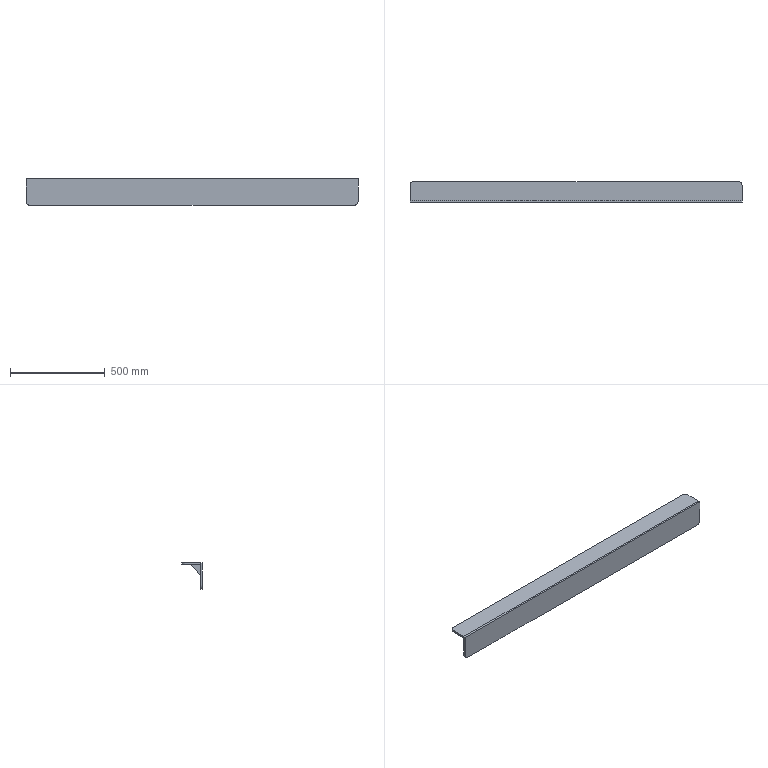Part | SolidWorks | features Fillet 2, ICE 2, Extrusion 1 | 3 solids | 21 faces | box 1748 x 110 x 139.4 mm | volume 4195006 mm3 | plane 17 | cylinder 4 | commonest cylinder face diameters 40 x4
STEP:
#1=CARTESIAN_POINT('',(873.75,0.,69.7));
#2=VERTEX_POINT('',#1);
#3=CARTESIAN_POINT('',(873.75,0.,-49.7));
#4=VERTEX_POINT('',#3);
#5=CARTESIAN_POINT('',(873.75,0.,-69.7));
#6=DIRECTION('',(0.,0.,-1.));
#7=VECTOR('',#6,1000.);
#8=LINE('',#5,#7);
#9=EDGE_CURVE('',#2,#4,#8,.T.);
#10=ORIENTED_EDGE('',*,*,#9,.T.);
#11=CARTESIAN_POINT('',(873.75,10.,-49.7));
#12=VERTEX_POINT('',#11);
#13=CARTESIAN_POINT('',(873.75,10.,-49.7));
#14=DIRECTION('',(0.,1.,0.));
#15=VECTOR('',#14,1000.);
#16=LINE('',#13,#15);
#17=EDGE_CURVE('',#4,#12,#16,.T.);
#18=ORIENTED_EDGE('',*,*,#17,.T.);
#19=CARTESIAN_POINT('',(873.75,10.,69.7));
#20=VERTEX_POINT('',#19);
#21=CARTESIAN_POINT('',(873.75,10.,-69.7));
#22=DIRECTION('',(0.,0.,-1.));
#23=VECTOR('',#22,1000.);
#24=LINE('',#21,#23);
#25=EDGE_CURVE('',#20,#12,#24,.T.);
#26=ORIENTED_EDGE('',*,*,#25,.F.);
#27=CARTESIAN_POINT('',(873.75,10.,69.7));
#28=DIRECTION('',(0.,-1.,0.));
#29=VECTOR('',#28,1000.);
#30=LINE('',#27,#29);
#31=EDGE_CURVE('',#20,#2,#30,.T.);
#32=ORIENTED_EDGE('',*,*,#31,.T.);
#33=EDGE_LOOP('',(#10,#18,#26,#32));
#34=FACE_OUTER_BOUND('',#33,.T.);
#35=CARTESIAN_POINT('',(873.75,10.,-69.7));
#36=DIRECTION('',(-1.,0.,0.));
#37=DIRECTION('',(0.,0.,1.));
#38=AXIS2_PLACEMENT_3D('',#35,#36,#37);
#39=PLANE('',#38);
#40=ADVANCED_FACE('',(#34),#39,.F.);
#41=CARTESIAN_POINT('',(853.75,0.,-69.7));
#42=VERTEX_POINT('',#41);
#43=CARTESIAN_POINT('',(-853.75,0.,-69.7));
#44=VERTEX_POINT('',#43);
#45=CARTESIAN_POINT('',(-873.75,0.,-69.7));
#46=DIRECTION('',(-1.,0.,0.));
#47=VECTOR('',#46,1000.);
#48=LINE('',#45,#47);
#49=EDGE_CURVE('',#42,#44,#48,.T.);
#50=ORIENTED_EDGE('',*,*,#49,.T.);
#51=CARTESIAN_POINT('',(-853.75,10.,-69.7));
#52=VERTEX_POINT('',#51);
#53=CARTESIAN_POINT('',(-853.75,10.,-69.7));
#54=DIRECTION('',(0.,1.,0.));
#55=VECTOR('',#54,1000.);
#56=LINE('',#53,#55);
#57=EDGE_CURVE('',#44,#52,#56,.T.);
#58=ORIENTED_EDGE('',*,*,#57,.T.);
#59=CARTESIAN_POINT('',(853.75,10.,-69.7));
#60=VERTEX_POINT('',#59);
#61=CARTESIAN_POINT('',(-873.75,10.,-69.7));
#62=DIRECTION('',(-1.,0.,0.));
#63=VECTOR('',#62,1000.);
#64=LINE('',#61,#63);
#65=EDGE_CURVE('',#60,#52,#64,.T.);
#66=ORIENTED_EDGE('',*,*,#65,.F.);
#67=CARTESIAN_POINT('',(853.75,10.,-69.7));
#68=DIRECTION('',(0.,-1.,0.));
#69=VECTOR('',#68,1000.);
#70=LINE('',#67,#69);
#71=EDGE_CURVE('',#60,#42,#70,.T.);
#72=ORIENTED_EDGE('',*,*,#71,.T.);
#73=EDGE_LOOP('',(#50,#58,#66,#72));
#74=FACE_OUTER_BOUND('',#73,.T.);
#75=CARTESIAN_POINT('',(-873.75,10.,-69.7));
#76=DIRECTION('',(0.,0.,1.));
#77=DIRECTION('',(1.,0.,0.));
#78=AXIS2_PLACEMENT_3D('',#75,#76,#77);
#79=PLANE('',#78);
#80=ADVANCED_FACE('',(#74),#79,.F.);
#81=CARTESIAN_POINT('',(-873.75,10.,-49.7));
#82=VERTEX_POINT('',#81);
#83=CARTESIAN_POINT('',(-873.75,10.,69.7));
#84=VERTEX_POINT('',#83);
#85=CARTESIAN_POINT('',(-873.75,10.,-69.7));
#86=DIRECTION('',(0.,0.,1.));
#87=VECTOR('',#86,1000.);
#88=LINE('',#85,#87);
#89=EDGE_CURVE('',#82,#84,#88,.T.);
#90=ORIENTED_EDGE('',*,*,#89,.F.);
#91=CARTESIAN_POINT('',(-873.75,0.,-49.7));
#92=VERTEX_POINT('',#91);
#93=CARTESIAN_POINT('',(-873.75,10.,-49.7));
#94=DIRECTION('',(0.,-1.,0.));
#95=VECTOR('',#94,1000.);
#96=LINE('',#93,#95);
#97=EDGE_CURVE('',#82,#92,#96,.T.);
#98=ORIENTED_EDGE('',*,*,#97,.T.);
#99=CARTESIAN_POINT('',(-873.75,0.,69.7));
#100=VERTEX_POINT('',#99);
#101=CARTESIAN_POINT('',(-873.75,0.,-69.7));
#102=DIRECTION('',(0.,0.,1.));
#103=VECTOR('',#102,1000.);
#104=LINE('',#101,#103);
#105=EDGE_CURVE('',#92,#100,#104,.T.);
#106=ORIENTED_EDGE('',*,*,#105,.T.);
#107=CARTESIAN_POINT('',(-873.75,10.,69.7));
#108=DIRECTION('',(0.,-1.,0.));
#109=VECTOR('',#108,1000.);
#110=LINE('',#107,#109);
#111=EDGE_CURVE('',#84,#100,#110,.T.);
#112=ORIENTED_EDGE('',*,*,#111,.F.);
#113=EDGE_LOOP('',(#90,#98,#106,#112));
#114=FACE_OUTER_BOUND('',#113,.T.);
#115=CARTESIAN_POINT('',(-873.75,10.,-69.7));
#116=DIRECTION('',(1.,0.,0.));
#117=DIRECTION('',(0.,0.,-1.));
#118=AXIS2_PLACEMENT_3D('',#115,#116,#117);
#119=PLANE('',#118);
#120=ADVANCED_FACE('',(#114),#119,.F.);
#121=CARTESIAN_POINT('',(-873.75,0.,69.7));
#122=DIRECTION('',(1.,0.,0.));
#123=VECTOR('',#122,1000.);
#124=LINE('',#121,#123);
#125=EDGE_CURVE('',#100,#2,#124,.T.);
#126=ORIENTED_EDGE('',*,*,#125,.T.);
#127=ORIENTED_EDGE('',*,*,#31,.F.);
#128=CARTESIAN_POINT('',(-873.75,10.,69.7));
#129=DIRECTION('',(1.,0.,0.));
#130=VECTOR('',#129,1000.);
#131=LINE('',#128,#130);
#132=EDGE_CURVE('',#84,#20,#131,.T.);
#133=ORIENTED_EDGE('',*,*,#132,.F.);
#134=ORIENTED_EDGE('',*,*,#111,.T.);
#135=EDGE_LOOP('',(#126,#127,#133,#134));
#136=FACE_OUTER_BOUND('',#135,.T.);
#137=CARTESIAN_POINT('',(-873.75,10.,69.7));
#138=DIRECTION('',(0.,0.,-1.));
#139=DIRECTION('',(-1.,0.,0.));
#140=AXIS2_PLACEMENT_3D('',#137,#138,#139);
#141=PLANE('',#140);
#142=ADVANCED_FACE('',(#136),#141,.F.);
#143=ORIENTED_EDGE('',*,*,#65,.T.);
#144=CARTESIAN_POINT('',(-853.75,10.,-49.7));
#145=DIRECTION('',(0.,1.,0.));
#146=DIRECTION('',(0.,0.,1.));
#147=AXIS2_PLACEMENT_3D('',#144,#145,#146);
#148=CIRCLE('',#147,20.);
#149=EDGE_CURVE('',#52,#82,#148,.T.);
#150=ORIENTED_EDGE('',*,*,#149,.T.);
#151=ORIENTED_EDGE('',*,*,#89,.T.);
#152=ORIENTED_EDGE('',*,*,#132,.T.);
#153=ORIENTED_EDGE('',*,*,#25,.T.);
#154=CARTESIAN_POINT('',(853.75,10.,-49.7));
#155=DIRECTION('',(0.,1.,0.));
#156=DIRECTION('',(0.,0.,1.));
#157=AXIS2_PLACEMENT_3D('',#154,#155,#156);
#158=CIRCLE('',#157,20.);
#159=EDGE_CURVE('',#12,#60,#158,.T.);
#160=ORIENTED_EDGE('',*,*,#159,.T.);
#161=EDGE_LOOP('',(#143,#150,#151,#152,#153,#160));
#162=FACE_OUTER_BOUND('',#161,.T.);
#163=CARTESIAN_POINT('',(0.,10.,0.));
#164=DIRECTION('',(0.,1.,0.));
#165=DIRECTION('',(0.,0.,1.));
#166=AXIS2_PLACEMENT_3D('',#163,#164,#165);
#167=PLANE('',#166);
#168=ADVANCED_FACE('',(#162),#167,.T.);
#169=ORIENTED_EDGE('',*,*,#105,.F.);
#170=CARTESIAN_POINT('',(-853.75,0.,-49.7));
#171=DIRECTION('',(0.,-1.,0.));
#172=DIRECTION('',(0.,0.,1.));
#173=AXIS2_PLACEMENT_3D('',#170,#171,#172);
#174=CIRCLE('',#173,20.);
#175=EDGE_CURVE('',#92,#44,#174,.T.);
#176=ORIENTED_EDGE('',*,*,#175,.T.);
#177=ORIENTED_EDGE('',*,*,#49,.F.);
#178=CARTESIAN_POINT('',(853.75,0.,-49.7));
#179=DIRECTION('',(0.,-1.,0.));
#180=DIRECTION('',(0.,0.,1.));
#181=AXIS2_PLACEMENT_3D('',#178,#179,#180);
#182=CIRCLE('',#181,20.);
#183=EDGE_CURVE('',#42,#4,#182,.T.);
#184=ORIENTED_EDGE('',*,*,#183,.T.);
#185=ORIENTED_EDGE('',*,*,#9,.F.);
#186=ORIENTED_EDGE('',*,*,#125,.F.);
#187=EDGE_LOOP('',(#169,#176,#177,#184,#185,#186));
#188=FACE_OUTER_BOUND('',#187,.T.);
#189=CARTESIAN_POINT('',(0.,0.,0.));
#190=DIRECTION('',(0.,1.,0.));
#191=DIRECTION('',(0.,0.,1.));
#192=AXIS2_PLACEMENT_3D('',#189,#190,#191);
#193=PLANE('',#192);
#194=ADVANCED_FACE('',(#188),#193,.F.);
#195=ORIENTED_EDGE('',*,*,#149,.F.);
#196=ORIENTED_EDGE('',*,*,#57,.F.);
#197=ORIENTED_EDGE('',*,*,#175,.F.);
#198=ORIENTED_EDGE('',*,*,#97,.F.);
#199=EDGE_LOOP('',(#195,#196,#197,#198));
#200=FACE_OUTER_BOUND('',#199,.T.);
#201=CARTESIAN_POINT('',(-853.75,10.,-49.7));
#202=DIRECTION('',(0.,-1.,0.));
#203=DIRECTION('',(0.,0.,-1.));
#204=AXIS2_PLACEMENT_3D('',#201,#202,#203);
#205=CYLINDRICAL_SURFACE('',#204,20.);
#206=ADVANCED_FACE('',(#200),#205,.T.);
#207=ORIENTED_EDGE('',*,*,#159,.F.);
#208=ORIENTED_EDGE('',*,*,#17,.F.);
#209=ORIENTED_EDGE('',*,*,#183,.F.);
#210=ORIENTED_EDGE('',*,*,#71,.F.);
#211=EDGE_LOOP('',(#207,#208,#209,#210));
#212=FACE_OUTER_BOUND('',#211,.T.);
#213=CARTESIAN_POINT('',(853.75,10.,-49.7));
#214=DIRECTION('',(0.,-1.,0.));
#215=DIRECTION('',(0.,0.,-1.));
#216=AXIS2_PLACEMENT_3D('',#213,#214,#215);
#217=CYLINDRICAL_SURFACE('',#216,20.);
#218=ADVANCED_FACE('',(#212),#217,.T.);
#219=CLOSED_SHELL('',(#40,#80,#120,#142,#168,#194,#206,#218));
#220=MANIFOLD_SOLID_BREP('',#219);
#221=CARTESIAN_POINT('',(-873.75,90.,69.7));
#222=VERTEX_POINT('',#221);
#223=CARTESIAN_POINT('',(-873.75,10.,69.7));
#224=VERTEX_POINT('',#223);
#225=CARTESIAN_POINT('',(-873.75,10.,69.7));
#226=DIRECTION('',(0.,-1.,0.));
#227=VECTOR('',#226,1000.);
#228=LINE('',#225,#227);
#229=EDGE_CURVE('',#222,#224,#228,.T.);
#230=ORIENTED_EDGE('',*,*,#229,.F.);
#231=CARTESIAN_POINT('',(-873.75,90.,59.7));
#232=VERTEX_POINT('',#231);
#233=CARTESIAN_POINT('',(-873.75,90.,59.7));
#234=DIRECTION('',(0.,0.,-1.));
#235=VECTOR('',#234,1000.);
#236=LINE('',#233,#235);
#237=EDGE_CURVE('',#222,#232,#236,.T.);
#238=ORIENTED_EDGE('',*,*,#237,.T.);
#239=CARTESIAN_POINT('',(-873.75,10.,59.7));
#240=VERTEX_POINT('',#239);
#241=CARTESIAN_POINT('',(-873.75,10.,59.7));
#242=DIRECTION('',(0.,-1.,0.));
#243=VECTOR('',#242,1000.);
#244=LINE('',#241,#243);
#245=EDGE_CURVE('',#232,#240,#244,.T.);
#246=ORIENTED_EDGE('',*,*,#245,.T.);
#247=CARTESIAN_POINT('',(-873.75,10.,59.7));
#248=DIRECTION('',(0.,0.,1.));
#249=VECTOR('',#248,1000.);
#250=LINE('',#247,#249);
#251=EDGE_CURVE('',#240,#224,#250,.T.);
#252=ORIENTED_EDGE('',*,*,#251,.T.);
#253=EDGE_LOOP('',(#230,#238,#246,#252));
#254=FACE_OUTER_BOUND('',#253,.T.);
#255=CARTESIAN_POINT('',(-873.75,10.,59.7));
#256=DIRECTION('',(-1.,0.,0.));
#257=DIRECTION('',(0.,0.,1.));
#258=AXIS2_PLACEMENT_3D('',#255,#256,#257);
#259=PLANE('',#258);
#260=ADVANCED_FACE('',(#254),#259,.T.);
#261=CARTESIAN_POINT('',(853.75,110.,69.7));
#262=VERTEX_POINT('',#261);
#263=CARTESIAN_POINT('',(-853.75,110.,69.7));
#264=VERTEX_POINT('',#263);
#265=CARTESIAN_POINT('',(-873.75,110.,69.7));
#266=DIRECTION('',(-1.,0.,0.));
#267=VECTOR('',#266,1000.);
#268=LINE('',#265,#267);
#269=EDGE_CURVE('',#262,#264,#268,.T.);
#270=ORIENTED_EDGE('',*,*,#269,.F.);
#271=CARTESIAN_POINT('',(853.75,110.,59.7));
#272=VERTEX_POINT('',#271);
#273=CARTESIAN_POINT('',(853.75,110.,59.7));
#274=DIRECTION('',(0.,0.,-1.));
#275=VECTOR('',#274,1000.);
#276=LINE('',#273,#275);
#277=EDGE_CURVE('',#262,#272,#276,.T.);
#278=ORIENTED_EDGE('',*,*,#277,.T.);
#279=CARTESIAN_POINT('',(-853.75,110.,59.7));
#280=VERTEX_POINT('',#279);
#281=CARTESIAN_POINT('',(-873.75,110.,59.7));
#282=DIRECTION('',(-1.,0.,0.));
#283=VECTOR('',#282,1000.);
#284=LINE('',#281,#283);
#285=EDGE_CURVE('',#272,#280,#284,.T.);
#286=ORIENTED_EDGE('',*,*,#285,.T.);
#287=CARTESIAN_POINT('',(-853.75,110.,59.7));
#288=DIRECTION('',(0.,0.,1.));
#289=VECTOR('',#288,1000.);
#290=LINE('',#287,#289);
#291=EDGE_CURVE('',#280,#264,#290,.T.);
#292=ORIENTED_EDGE('',*,*,#291,.T.);
#293=EDGE_LOOP('',(#270,#278,#286,#292));
#294=FACE_OUTER_BOUND('',#293,.T.);
#295=CARTESIAN_POINT('',(-873.75,110.,59.7));
#296=DIRECTION('',(0.,1.,0.));
#297=DIRECTION('',(0.,0.,1.));
#298=AXIS2_PLACEMENT_3D('',#295,#296,#297);
#299=PLANE('',#298);
#300=ADVANCED_FACE('',(#294),#299,.T.);
#301=CARTESIAN_POINT('',(873.75,10.,59.7));
#302=VERTEX_POINT('',#301);
#303=CARTESIAN_POINT('',(873.75,90.,59.7));
#304=VERTEX_POINT('',#303);
#305=CARTESIAN_POINT('',(873.75,10.,59.7));
#306=DIRECTION('',(0.,1.,0.));
#307=VECTOR('',#306,1000.);
#308=LINE('',#305,#307);
#309=EDGE_CURVE('',#302,#304,#308,.T.);
#310=ORIENTED_EDGE('',*,*,#309,.T.);
#311=CARTESIAN_POINT('',(873.75,90.,69.7));
#312=VERTEX_POINT('',#311);
#313=CARTESIAN_POINT('',(873.75,90.,59.7));
#314=DIRECTION('',(0.,0.,1.));
#315=VECTOR('',#314,1000.);
#316=LINE('',#313,#315);
#317=EDGE_CURVE('',#304,#312,#316,.T.);
#318=ORIENTED_EDGE('',*,*,#317,.T.);
#319=CARTESIAN_POINT('',(873.75,10.,69.7));
#320=VERTEX_POINT('',#319);
#321=CARTESIAN_POINT('',(873.75,10.,69.7));
#322=DIRECTION('',(0.,1.,0.));
#323=VECTOR('',#322,1000.);
#324=LINE('',#321,#323);
#325=EDGE_CURVE('',#320,#312,#324,.T.);
#326=ORIENTED_EDGE('',*,*,#325,.F.);
#327=CARTESIAN_POINT('',(873.75,10.,59.7));
#328=DIRECTION('',(0.,0.,1.));
#329=VECTOR('',#328,1000.);
#330=LINE('',#327,#329);
#331=EDGE_CURVE('',#302,#320,#330,.T.);
#332=ORIENTED_EDGE('',*,*,#331,.F.);
#333=EDGE_LOOP('',(#310,#318,#326,#332));
#334=FACE_OUTER_BOUND('',#333,.T.);
#335=CARTESIAN_POINT('',(873.75,10.,59.7));
#336=DIRECTION('',(1.,0.,0.));
#337=DIRECTION('',(0.,0.,-1.));
#338=AXIS2_PLACEMENT_3D('',#335,#336,#337);
#339=PLANE('',#338);
#340=ADVANCED_FACE('',(#334),#339,.T.);
#341=CARTESIAN_POINT('',(-873.75,10.,69.7));
#342=DIRECTION('',(1.,0.,0.));
#343=VECTOR('',#342,1000.);
#344=LINE('',#341,#343);
#345=EDGE_CURVE('',#224,#320,#344,.T.);
#346=ORIENTED_EDGE('',*,*,#345,.F.);
#347=ORIENTED_EDGE('',*,*,#251,.F.);
#348=CARTESIAN_POINT('',(-873.75,10.,59.7));
#349=DIRECTION('',(1.,0.,0.));
#350=VECTOR('',#349,1000.);
#351=LINE('',#348,#350);
#352=EDGE_CURVE('',#240,#302,#351,.T.);
#353=ORIENTED_EDGE('',*,*,#352,.T.);
#354=ORIENTED_EDGE('',*,*,#331,.T.);
#355=EDGE_LOOP('',(#346,#347,#353,#354));
#356=FACE_OUTER_BOUND('',#355,.T.);
#357=CARTESIAN_POINT('',(-873.75,10.,59.7));
#358=DIRECTION('',(0.,-1.,0.));
#359=DIRECTION('',(0.,0.,-1.));
#360=AXIS2_PLACEMENT_3D('',#357,#358,#359);
#361=PLANE('',#360);
#362=ADVANCED_FACE('',(#356),#361,.T.);
#363=ORIENTED_EDGE('',*,*,#285,.F.);
#364=CARTESIAN_POINT('',(853.75,90.,59.7));
#365=DIRECTION('',(0.,0.,-1.));
#366=DIRECTION('',(-1.,0.,0.));
#367=AXIS2_PLACEMENT_3D('',#364,#365,#366);
#368=CIRCLE('',#367,20.);
#369=EDGE_CURVE('',#272,#304,#368,.T.);
#370=ORIENTED_EDGE('',*,*,#369,.T.);
#371=ORIENTED_EDGE('',*,*,#309,.F.);
#372=ORIENTED_EDGE('',*,*,#352,.F.);
#373=ORIENTED_EDGE('',*,*,#245,.F.);
#374=CARTESIAN_POINT('',(-853.75,90.,59.7));
#375=DIRECTION('',(0.,0.,-1.));
#376=DIRECTION('',(-1.,0.,0.));
#377=AXIS2_PLACEMENT_3D('',#374,#375,#376);
#378=CIRCLE('',#377,20.);
#379=EDGE_CURVE('',#232,#280,#378,.T.);
#380=ORIENTED_EDGE('',*,*,#379,.T.);
#381=EDGE_LOOP('',(#363,#370,#371,#372,#373,#380));
#382=FACE_OUTER_BOUND('',#381,.T.);
#383=CARTESIAN_POINT('',(0.,0.,59.7));
#384=DIRECTION('',(0.,0.,-1.));
#385=DIRECTION('',(-1.,0.,0.));
#386=AXIS2_PLACEMENT_3D('',#383,#384,#385);
#387=PLANE('',#386);
#388=ADVANCED_FACE('',(#382),#387,.T.);
#389=ORIENTED_EDGE('',*,*,#325,.T.);
#390=CARTESIAN_POINT('',(853.75,90.,69.7));
#391=DIRECTION('',(0.,0.,1.));
#392=DIRECTION('',(-1.,0.,0.));
#393=AXIS2_PLACEMENT_3D('',#390,#391,#392);
#394=CIRCLE('',#393,20.);
#395=EDGE_CURVE('',#312,#262,#394,.T.);
#396=ORIENTED_EDGE('',*,*,#395,.T.);
#397=ORIENTED_EDGE('',*,*,#269,.T.);
#398=CARTESIAN_POINT('',(-853.75,90.,69.7));
#399=DIRECTION('',(0.,0.,1.));
#400=DIRECTION('',(-1.,0.,0.));
#401=AXIS2_PLACEMENT_3D('',#398,#399,#400);
#402=CIRCLE('',#401,20.);
#403=EDGE_CURVE('',#264,#222,#402,.T.);
#404=ORIENTED_EDGE('',*,*,#403,.T.);
#405=ORIENTED_EDGE('',*,*,#229,.T.);
#406=ORIENTED_EDGE('',*,*,#345,.T.);
#407=EDGE_LOOP('',(#389,#396,#397,#404,#405,#406));
#408=FACE_OUTER_BOUND('',#407,.T.);
#409=CARTESIAN_POINT('',(0.,0.,69.7));
#410=DIRECTION('',(0.,0.,-1.));
#411=DIRECTION('',(-1.,0.,0.));
#412=AXIS2_PLACEMENT_3D('',#409,#410,#411);
#413=PLANE('',#412);
#414=ADVANCED_FACE('',(#408),#413,.F.);
#415=ORIENTED_EDGE('',*,*,#369,.F.);
#416=ORIENTED_EDGE('',*,*,#277,.F.);
#417=ORIENTED_EDGE('',*,*,#395,.F.);
#418=ORIENTED_EDGE('',*,*,#317,.F.);
#419=EDGE_LOOP('',(#415,#416,#417,#418));
#420=FACE_OUTER_BOUND('',#419,.T.);
#421=CARTESIAN_POINT('',(853.75,90.,59.7));
#422=DIRECTION('',(0.,0.,1.));
#423=DIRECTION('',(1.,0.,0.));
#424=AXIS2_PLACEMENT_3D('',#421,#422,#423);
#425=CYLINDRICAL_SURFACE('',#424,20.);
#426=ADVANCED_FACE('',(#420),#425,.T.);
#427=ORIENTED_EDGE('',*,*,#379,.F.);
#428=ORIENTED_EDGE('',*,*,#237,.F.);
#429=ORIENTED_EDGE('',*,*,#403,.F.);
#430=ORIENTED_EDGE('',*,*,#291,.F.);
#431=EDGE_LOOP('',(#427,#428,#429,#430));
#432=FACE_OUTER_BOUND('',#431,.T.);
#433=CARTESIAN_POINT('',(-853.75,90.,59.7));
#434=DIRECTION('',(0.,0.,1.));
#435=DIRECTION('',(1.,0.,0.));
#436=AXIS2_PLACEMENT_3D('',#433,#434,#435);
#437=CYLINDRICAL_SURFACE('',#436,20.);
#438=ADVANCED_FACE('',(#432),#437,.T.);
#439=CLOSED_SHELL('',(#260,#300,#340,#362,#388,#414,#426,#438));
#440=MANIFOLD_SOLID_BREP('',#439);
#441=CARTESIAN_POINT('',(-5.,10.,59.7));
#442=VERTEX_POINT('',#441);
#443=CARTESIAN_POINT('',(-5.,10.,0.));
#444=VERTEX_POINT('',#443);
#445=CARTESIAN_POINT('',(-5.,10.,59.7));
#446=DIRECTION('',(0.,0.,-1.));
#447=VECTOR('',#446,1000.);
#448=LINE('',#445,#447);
#449=EDGE_CURVE('',#442,#444,#448,.T.);
#450=ORIENTED_EDGE('',*,*,#449,.T.);
#451=CARTESIAN_POINT('',(5.,10.,0.));
#452=VERTEX_POINT('',#451);
#453=CARTESIAN_POINT('',(5.,10.,0.));
#454=DIRECTION('',(-1.,0.,0.));
#455=VECTOR('',#454,1000.);
#456=LINE('',#453,#455);
#457=EDGE_CURVE('',#452,#444,#456,.T.);
#458=ORIENTED_EDGE('',*,*,#457,.F.);
#459=CARTESIAN_POINT('',(5.,10.,59.7));
#460=VERTEX_POINT('',#459);
#461=CARTESIAN_POINT('',(5.,10.,59.7));
#462=DIRECTION('',(0.,0.,-1.));
#463=VECTOR('',#462,1000.);
#464=LINE('',#461,#463);
#465=EDGE_CURVE('',#460,#452,#464,.T.);
#466=ORIENTED_EDGE('',*,*,#465,.F.);
#467=CARTESIAN_POINT('',(5.,10.,59.7));
#468=DIRECTION('',(-1.,0.,0.));
#469=VECTOR('',#468,1000.);
#470=LINE('',#467,#469);
#471=EDGE_CURVE('',#460,#442,#470,.T.);
#472=ORIENTED_EDGE('',*,*,#471,.T.);
#473=EDGE_LOOP('',(#450,#458,#466,#472));
#474=FACE_OUTER_BOUND('',#473,.T.);
#475=CARTESIAN_POINT('',(5.,10.,59.7));
#476=DIRECTION('',(0.,1.,0.));
#477=DIRECTION('',(0.,0.,1.));
#478=AXIS2_PLACEMENT_3D('',#475,#476,#477);
#479=PLANE('',#478);
#480=ADVANCED_FACE('',(#474),#479,.F.);
#481=CARTESIAN_POINT('',(-5.,60.,59.7));
#482=VERTEX_POINT('',#481);
#483=CARTESIAN_POINT('',(-5.,10.,0.));
#484=DIRECTION('',(0.,0.6421,0.7666));
#485=VECTOR('',#484,1000.);
#486=LINE('',#483,#485);
#487=EDGE_CURVE('',#444,#482,#486,.T.);
#488=ORIENTED_EDGE('',*,*,#487,.T.);
#489=CARTESIAN_POINT('',(5.,60.,59.7));
#490=VERTEX_POINT('',#489);
#491=CARTESIAN_POINT('',(5.,60.,59.7));
#492=DIRECTION('',(-1.,0.,0.));
#493=VECTOR('',#492,1000.);
#494=LINE('',#491,#493);
#495=EDGE_CURVE('',#490,#482,#494,.T.);
#496=ORIENTED_EDGE('',*,*,#495,.F.);
#497=CARTESIAN_POINT('',(5.,10.,0.));
#498=DIRECTION('',(0.,0.6421,0.7666));
#499=VECTOR('',#498,1000.);
#500=LINE('',#497,#499);
#501=EDGE_CURVE('',#452,#490,#500,.T.);
#502=ORIENTED_EDGE('',*,*,#501,.F.);
#503=ORIENTED_EDGE('',*,*,#457,.T.);
#504=EDGE_LOOP('',(#488,#496,#502,#503));
#505=FACE_OUTER_BOUND('',#504,.T.);
#506=CARTESIAN_POINT('',(5.,10.,0.));
#507=DIRECTION('',(0.,-0.7666,0.6421));
#508=DIRECTION('',(0.,-0.6421,-0.7666));
#509=AXIS2_PLACEMENT_3D('',#506,#507,#508);
#510=PLANE('',#509);
#511=ADVANCED_FACE('',(#505),#510,.F.);
#512=CARTESIAN_POINT('',(-5.,60.,59.7));
#513=DIRECTION('',(0.,-1.,0.));
#514=VECTOR('',#513,1000.);
#515=LINE('',#512,#514);
#516=EDGE_CURVE('',#482,#442,#515,.T.);
#517=ORIENTED_EDGE('',*,*,#516,.T.);
#518=ORIENTED_EDGE('',*,*,#471,.F.);
#519=CARTESIAN_POINT('',(5.,60.,59.7));
#520=DIRECTION('',(0.,-1.,0.));
#521=VECTOR('',#520,1000.);
#522=LINE('',#519,#521);
#523=EDGE_CURVE('',#490,#460,#522,.T.);
#524=ORIENTED_EDGE('',*,*,#523,.F.);
#525=ORIENTED_EDGE('',*,*,#495,.T.);
#526=EDGE_LOOP('',(#517,#518,#524,#525));
#527=FACE_OUTER_BOUND('',#526,.T.);
#528=CARTESIAN_POINT('',(5.,60.,59.7));
#529=DIRECTION('',(0.,0.,-1.));
#530=DIRECTION('',(-1.,0.,0.));
#531=AXIS2_PLACEMENT_3D('',#528,#529,#530);
#532=PLANE('',#531);
#533=ADVANCED_FACE('',(#527),#532,.F.);
#534=ORIENTED_EDGE('',*,*,#465,.T.);
#535=ORIENTED_EDGE('',*,*,#501,.T.);
#536=ORIENTED_EDGE('',*,*,#523,.T.);
#537=EDGE_LOOP('',(#534,#535,#536));
#538=FACE_OUTER_BOUND('',#537,.T.);
#539=CARTESIAN_POINT('',(5.,0.,0.));
#540=DIRECTION('',(-1.,0.,0.));
#541=DIRECTION('',(0.,0.,1.));
#542=AXIS2_PLACEMENT_3D('',#539,#540,#541);
#543=PLANE('',#542);
#544=ADVANCED_FACE('',(#538),#543,.F.);
#545=ORIENTED_EDGE('',*,*,#449,.F.);
#546=ORIENTED_EDGE('',*,*,#516,.F.);
#547=ORIENTED_EDGE('',*,*,#487,.F.);
#548=EDGE_LOOP('',(#545,#546,#547));
#549=FACE_OUTER_BOUND('',#548,.T.);
#550=CARTESIAN_POINT('',(-5.,0.,0.));
#551=DIRECTION('',(-1.,0.,0.));
#552=DIRECTION('',(0.,0.,1.));
#553=AXIS2_PLACEMENT_3D('',#550,#551,#552);
#554=PLANE('',#553);
#555=ADVANCED_FACE('',(#549),#554,.T.);
#556=CLOSED_SHELL('',(#480,#511,#533,#544,#555));
#557=MANIFOLD_SOLID_BREP('',#556);
#558=CARTESIAN_POINT('',(0.,0.,0.));
#559=DIRECTION('',(0.,0.,1.));
#560=DIRECTION('',(1.,0.,0.));
#561=AXIS2_PLACEMENT_3D('',#558,#559,#560);
#562=(LENGTH_UNIT()NAMED_UNIT(*)SI_UNIT(.MILLI.,.METRE.));
#563=UNCERTAINTY_MEASURE_WITH_UNIT(LENGTH_MEASURE(0.00001),#562,'','');
#564=(NAMED_UNIT(*)PLANE_ANGLE_UNIT()SI_UNIT($,.RADIAN.));
#565=(NAMED_UNIT(*)SI_UNIT($,.STERADIAN.)SOLID_ANGLE_UNIT());
#566=(GEOMETRIC_REPRESENTATION_CONTEXT(3)GLOBAL_UNCERTAINTY_ASSIGNED_CONTEXT((#563))GLOBAL_UNIT_ASSIGNED_CONTEXT((#562,#564,#565))REPRESENTATION_CONTEXT('',''));
#567=ADVANCED_BREP_SHAPE_REPRESENTATION('',(#220,#440,#557,#561),#566);